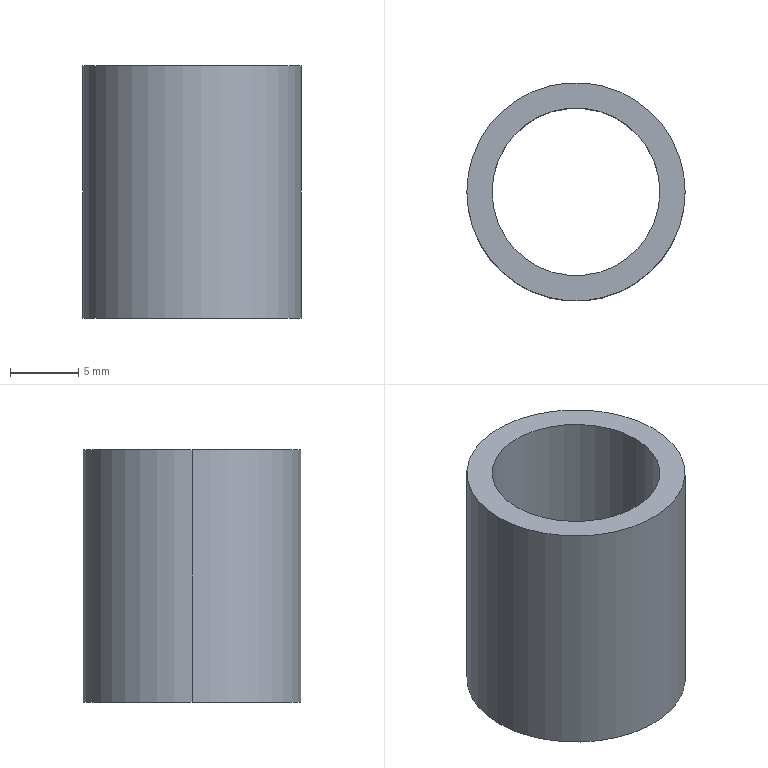Part | SolidWorks | features Extrusion 1 | 1 solid | 6 faces | box 16 x 16 x 18.5 mm | volume 1521 mm3 | cylinder 4 | plane 2 | commonest cylinder face diameters 12.3 x2 16 x2
STEP:
#1=CARTESIAN_POINT('',(93.85,71.3,18.5));
#2=VERTEX_POINT('',#1);
#3=CARTESIAN_POINT('',(106.15,71.3,18.5));
#4=VERTEX_POINT('',#3);
#5=CARTESIAN_POINT('',(100.,71.3,18.5));
#6=DIRECTION('',(0.,0.,1.));
#7=DIRECTION('',(1.,0.,0.));
#8=AXIS2_PLACEMENT_3D('',#5,#6,#7);
#9=CIRCLE('',#8,6.15);
#10=EDGE_CURVE('',#2,#4,#9,.T.);
#11=ORIENTED_EDGE('',*,*,#10,.T.);
#12=CARTESIAN_POINT('',(106.15,71.3,0.));
#13=VERTEX_POINT('',#12);
#14=CARTESIAN_POINT('',(106.15,71.3,41.127));
#15=DIRECTION('',(0.,0.,-1.));
#16=VECTOR('',#15,1000.);
#17=LINE('',#14,#16);
#18=EDGE_CURVE('',#4,#13,#17,.T.);
#19=ORIENTED_EDGE('',*,*,#18,.T.);
#20=CARTESIAN_POINT('',(93.85,71.3,0.));
#21=VERTEX_POINT('',#20);
#22=CARTESIAN_POINT('',(100.,71.3,0.));
#23=DIRECTION('',(0.,0.,1.));
#24=DIRECTION('',(1.,0.,0.));
#25=AXIS2_PLACEMENT_3D('',#22,#23,#24);
#26=CIRCLE('',#25,6.15);
#27=EDGE_CURVE('',#21,#13,#26,.T.);
#28=ORIENTED_EDGE('',*,*,#27,.F.);
#29=CARTESIAN_POINT('',(93.85,71.3,41.127));
#30=DIRECTION('',(0.,0.,-1.));
#31=VECTOR('',#30,1000.);
#32=LINE('',#29,#31);
#33=EDGE_CURVE('',#2,#21,#32,.T.);
#34=ORIENTED_EDGE('',*,*,#33,.F.);
#35=EDGE_LOOP('',(#11,#19,#28,#34));
#36=FACE_OUTER_BOUND('',#35,.T.);
#37=CARTESIAN_POINT('',(100.,71.3,41.127));
#38=DIRECTION('',(0.,0.,-1.));
#39=DIRECTION('',(-1.,0.,0.));
#40=AXIS2_PLACEMENT_3D('',#37,#38,#39);
#41=CYLINDRICAL_SURFACE('',#40,6.15);
#42=ADVANCED_FACE('',(#36),#41,.F.);
#43=CARTESIAN_POINT('',(108.,71.3,18.5));
#44=VERTEX_POINT('',#43);
#45=CARTESIAN_POINT('',(92.,71.3,18.5));
#46=VERTEX_POINT('',#45);
#47=CARTESIAN_POINT('',(100.,71.3,18.5));
#48=DIRECTION('',(0.,0.,1.));
#49=DIRECTION('',(1.,0.,0.));
#50=AXIS2_PLACEMENT_3D('',#47,#48,#49);
#51=CIRCLE('',#50,8.);
#52=EDGE_CURVE('',#44,#46,#51,.T.);
#53=ORIENTED_EDGE('',*,*,#52,.F.);
#54=CARTESIAN_POINT('',(108.,71.3,0.));
#55=VERTEX_POINT('',#54);
#56=CARTESIAN_POINT('',(108.,71.3,41.127));
#57=DIRECTION('',(0.,0.,-1.));
#58=VECTOR('',#57,1000.);
#59=LINE('',#56,#58);
#60=EDGE_CURVE('',#44,#55,#59,.T.);
#61=ORIENTED_EDGE('',*,*,#60,.T.);
#62=CARTESIAN_POINT('',(92.,71.3,0.));
#63=VERTEX_POINT('',#62);
#64=CARTESIAN_POINT('',(100.,71.3,0.));
#65=DIRECTION('',(0.,0.,1.));
#66=DIRECTION('',(1.,0.,0.));
#67=AXIS2_PLACEMENT_3D('',#64,#65,#66);
#68=CIRCLE('',#67,8.);
#69=EDGE_CURVE('',#55,#63,#68,.T.);
#70=ORIENTED_EDGE('',*,*,#69,.T.);
#71=CARTESIAN_POINT('',(92.,71.3,41.127));
#72=DIRECTION('',(0.,0.,-1.));
#73=VECTOR('',#72,1000.);
#74=LINE('',#71,#73);
#75=EDGE_CURVE('',#46,#63,#74,.T.);
#76=ORIENTED_EDGE('',*,*,#75,.F.);
#77=EDGE_LOOP('',(#53,#61,#70,#76));
#78=FACE_OUTER_BOUND('',#77,.T.);
#79=CARTESIAN_POINT('',(100.,71.3,41.127));
#80=DIRECTION('',(0.,0.,-1.));
#81=DIRECTION('',(-1.,0.,0.));
#82=AXIS2_PLACEMENT_3D('',#79,#80,#81);
#83=CYLINDRICAL_SURFACE('',#82,8.);
#84=ADVANCED_FACE('',(#78),#83,.T.);
#85=ORIENTED_EDGE('',*,*,#60,.F.);
#86=CARTESIAN_POINT('',(100.,71.3,18.5));
#87=DIRECTION('',(0.,0.,1.));
#88=DIRECTION('',(1.,0.,0.));
#89=AXIS2_PLACEMENT_3D('',#86,#87,#88);
#90=CIRCLE('',#89,8.);
#91=EDGE_CURVE('',#46,#44,#90,.T.);
#92=ORIENTED_EDGE('',*,*,#91,.F.);
#93=ORIENTED_EDGE('',*,*,#75,.T.);
#94=CARTESIAN_POINT('',(100.,71.3,0.));
#95=DIRECTION('',(0.,0.,1.));
#96=DIRECTION('',(1.,0.,0.));
#97=AXIS2_PLACEMENT_3D('',#94,#95,#96);
#98=CIRCLE('',#97,8.);
#99=EDGE_CURVE('',#63,#55,#98,.T.);
#100=ORIENTED_EDGE('',*,*,#99,.T.);
#101=EDGE_LOOP('',(#85,#92,#93,#100));
#102=FACE_OUTER_BOUND('',#101,.T.);
#103=CARTESIAN_POINT('',(100.,71.3,41.127));
#104=DIRECTION('',(0.,0.,-1.));
#105=DIRECTION('',(-1.,0.,0.));
#106=AXIS2_PLACEMENT_3D('',#103,#104,#105);
#107=CYLINDRICAL_SURFACE('',#106,8.);
#108=ADVANCED_FACE('',(#102),#107,.T.);
#109=ORIENTED_EDGE('',*,*,#99,.F.);
#110=ORIENTED_EDGE('',*,*,#69,.F.);
#111=EDGE_LOOP('',(#109,#110));
#112=FACE_OUTER_BOUND('',#111,.T.);
#113=ORIENTED_EDGE('',*,*,#27,.T.);
#114=CARTESIAN_POINT('',(100.,71.3,0.));
#115=DIRECTION('',(0.,0.,1.));
#116=DIRECTION('',(1.,0.,0.));
#117=AXIS2_PLACEMENT_3D('',#114,#115,#116);
#118=CIRCLE('',#117,6.15);
#119=EDGE_CURVE('',#13,#21,#118,.T.);
#120=ORIENTED_EDGE('',*,*,#119,.T.);
#121=EDGE_LOOP('',(#113,#120));
#122=FACE_BOUND('',#121,.T.);
#123=CARTESIAN_POINT('',(100.,71.3,0.));
#124=DIRECTION('',(0.,0.,1.));
#125=DIRECTION('',(1.,0.,0.));
#126=AXIS2_PLACEMENT_3D('',#123,#124,#125);
#127=PLANE('',#126);
#128=ADVANCED_FACE('',(#112,#122),#127,.F.);
#129=ORIENTED_EDGE('',*,*,#18,.F.);
#130=CARTESIAN_POINT('',(100.,71.3,18.5));
#131=DIRECTION('',(0.,0.,1.));
#132=DIRECTION('',(1.,0.,0.));
#133=AXIS2_PLACEMENT_3D('',#130,#131,#132);
#134=CIRCLE('',#133,6.15);
#135=EDGE_CURVE('',#4,#2,#134,.T.);
#136=ORIENTED_EDGE('',*,*,#135,.T.);
#137=ORIENTED_EDGE('',*,*,#33,.T.);
#138=ORIENTED_EDGE('',*,*,#119,.F.);
#139=EDGE_LOOP('',(#129,#136,#137,#138));
#140=FACE_OUTER_BOUND('',#139,.T.);
#141=CARTESIAN_POINT('',(100.,71.3,41.127));
#142=DIRECTION('',(0.,0.,-1.));
#143=DIRECTION('',(-1.,0.,0.));
#144=AXIS2_PLACEMENT_3D('',#141,#142,#143);
#145=CYLINDRICAL_SURFACE('',#144,6.15);
#146=ADVANCED_FACE('',(#140),#145,.F.);
#147=ORIENTED_EDGE('',*,*,#10,.F.);
#148=ORIENTED_EDGE('',*,*,#135,.F.);
#149=EDGE_LOOP('',(#147,#148));
#150=FACE_BOUND('',#149,.T.);
#151=ORIENTED_EDGE('',*,*,#91,.T.);
#152=ORIENTED_EDGE('',*,*,#52,.T.);
#153=EDGE_LOOP('',(#151,#152));
#154=FACE_OUTER_BOUND('',#153,.T.);
#155=CARTESIAN_POINT('',(113.,93.3,18.5));
#156=DIRECTION('',(0.,0.,1.));
#157=DIRECTION('',(0.,1.,0.));
#158=AXIS2_PLACEMENT_3D('',#155,#156,#157);
#159=PLANE('',#158);
#160=ADVANCED_FACE('',(#150,#154),#159,.T.);
#161=CLOSED_SHELL('',(#42,#84,#108,#128,#146,#160));
#162=MANIFOLD_SOLID_BREP('',#161);
#163=CARTESIAN_POINT('',(0.,0.,0.));
#164=DIRECTION('',(0.,0.,1.));
#165=DIRECTION('',(1.,0.,0.));
#166=AXIS2_PLACEMENT_3D('',#163,#164,#165);
#167=(LENGTH_UNIT()NAMED_UNIT(*)SI_UNIT(.MILLI.,.METRE.));
#168=UNCERTAINTY_MEASURE_WITH_UNIT(LENGTH_MEASURE(0.00001),#167,'','');
#169=(NAMED_UNIT(*)PLANE_ANGLE_UNIT()SI_UNIT($,.RADIAN.));
#170=(NAMED_UNIT(*)SI_UNIT($,.STERADIAN.)SOLID_ANGLE_UNIT());
#171=(GEOMETRIC_REPRESENTATION_CONTEXT(3)GLOBAL_UNCERTAINTY_ASSIGNED_CONTEXT((#168))GLOBAL_UNIT_ASSIGNED_CONTEXT((#167,#169,#170))REPRESENTATION_CONTEXT('',''));
#172=ADVANCED_BREP_SHAPE_REPRESENTATION('',(#162,#166),#171);